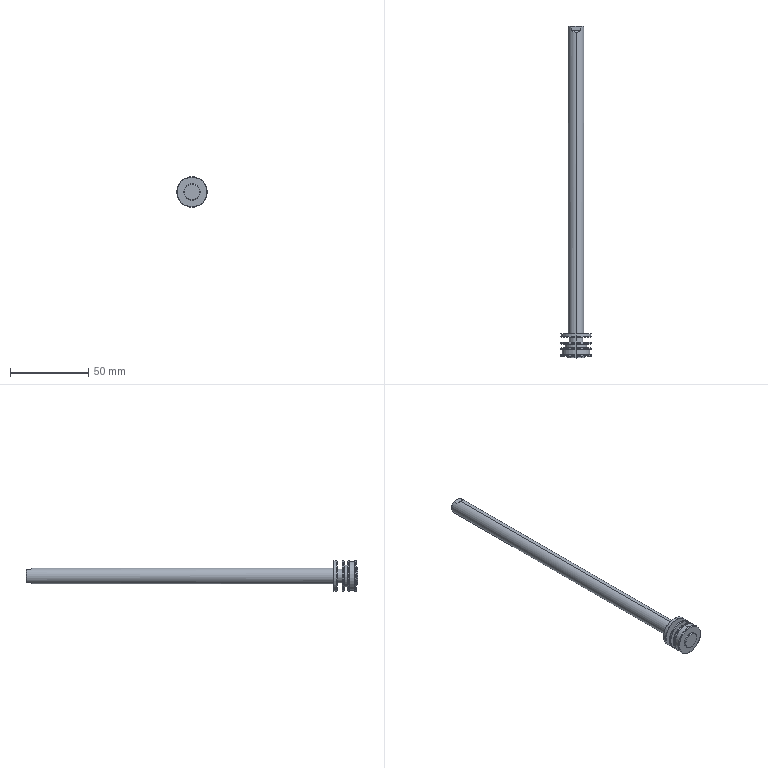Part | SolidWorks | features BaseBody 1 | 1 solid | 59 faces | box 19.6 x 212.6 x 19.6 mm | volume 18401 mm3 | cylinder 21 | cone 20 | plane 14 | torus 4 | commonest cylinder face diameters 19.6 x8 4.917 x3 8.8 x2 10 x2 10.6 x2 14 x2